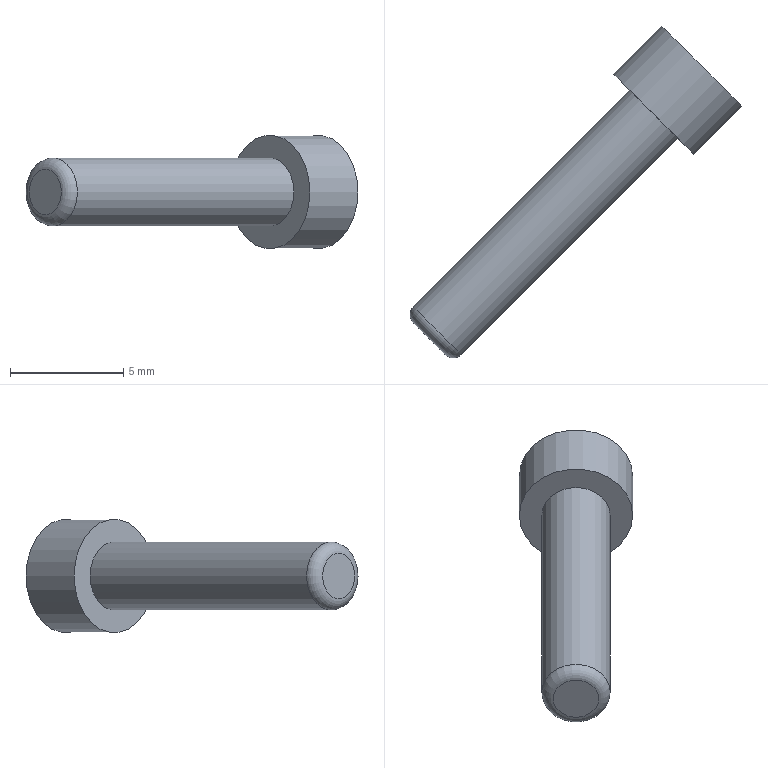Part | STEP file | gslz 2016.10.28-13_id650_x_t | 1 solid | 6 faces | box 14.642 x 14.642 x 5 mm | volume 157.397 mm3 | plane 3 | cylinder 2 | torus 1 | commonest cylinder face diameters 3 x1 5 x1
STEP:
#1=CARTESIAN_POINT('',(0.,0.,0.));
#2=DIRECTION('',(0.,0.,1.));
#3=DIRECTION('',(1.,0.,0.));
#4=AXIS2_PLACEMENT_3D('',#1,#2,#3);
#5=CARTESIAN_POINT('',(550.913,157.257,-21.226));
#6=VERTEX_POINT('',#5);
#7=CARTESIAN_POINT('',(551.974,156.197,-21.226));
#8=DIRECTION('',(0.7071,0.7071,0.));
#9=DIRECTION('',(-0.7071,0.7071,0.));
#10=AXIS2_PLACEMENT_3D('',#7,#8,#9);
#11=CIRCLE('',#10,1.5);
#12=CARTESIAN_POINT('',(552.328,156.55,-21.226));
#13=DIRECTION('',(0.7071,0.7071,0.));
#14=DIRECTION('',(-0.7071,0.7071,0.));
#15=AXIS2_PLACEMENT_3D('',#12,#13,#14);
#16=CYLINDRICAL_SURFACE('',#15,1.5);
#17=CARTESIAN_POINT('',(0.,-0.5));
#18=DIRECTION('',(1.,0.));
#19=VECTOR('',#18,1.);
#20=LINE('',#17,#19);
#21=(GEOMETRIC_REPRESENTATION_CONTEXT(2)PARAMETRIC_REPRESENTATION_CONTEXT()REPRESENTATION_CONTEXT('',''));
#22=DEFINITIONAL_REPRESENTATION('',(#20),#21);
#23=PCURVE('',#16,#22);
#24=CARTESIAN_POINT('',(551.974,156.197,-21.226));
#25=DIRECTION('',(0.7071,0.7071,0.));
#26=DIRECTION('',(-0.7071,0.7071,0.));
#27=AXIS2_PLACEMENT_3D('',#24,#25,#26);
#28=TOROIDAL_SURFACE('',#27,1.,0.5);
#29=CARTESIAN_POINT('',(0.,6.283));
#30=DIRECTION('',(1.,0.));
#31=VECTOR('',#30,1.);
#32=LINE('',#29,#31);
#33=(GEOMETRIC_REPRESENTATION_CONTEXT(2)PARAMETRIC_REPRESENTATION_CONTEXT()REPRESENTATION_CONTEXT('',''));
#34=DEFINITIONAL_REPRESENTATION('',(#32),#33);
#35=PCURVE('',#28,#34);
#36=SURFACE_CURVE('',#11,(#23,#35),.PCURVE_S1.);
#37=EDGE_CURVE('',#6,#6,#36,.T.);
#38=ORIENTED_EDGE('',*,*,#37,.T.);
#39=CARTESIAN_POINT('',(560.459,166.803,-21.226));
#40=VERTEX_POINT('',#39);
#41=CARTESIAN_POINT('',(550.913,157.257,-21.226));
#42=CARTESIAN_POINT('',(560.459,166.803,-21.226));
#43=B_SPLINE_CURVE_WITH_KNOTS('',1,(#41,#42),.UNSPECIFIED.,.F.,.F.,(2,2),(-0.5,13.),.PIECEWISE_BEZIER_KNOTS.);
#44=CARTESIAN_POINT('',(6.283,0.));
#45=DIRECTION('',(0.,1.));
#46=VECTOR('',#45,1.);
#47=LINE('',#44,#46);
#48=(GEOMETRIC_REPRESENTATION_CONTEXT(2)PARAMETRIC_REPRESENTATION_CONTEXT()REPRESENTATION_CONTEXT('',''));
#49=DEFINITIONAL_REPRESENTATION('',(#47),#48);
#50=PCURVE('',#16,#49);
#51=CARTESIAN_POINT('',(0.,0.));
#52=DIRECTION('',(0.,1.));
#53=VECTOR('',#52,1.);
#54=LINE('',#51,#53);
#55=(GEOMETRIC_REPRESENTATION_CONTEXT(2)PARAMETRIC_REPRESENTATION_CONTEXT()REPRESENTATION_CONTEXT('',''));
#56=DEFINITIONAL_REPRESENTATION('',(#54),#55);
#57=PCURVE('',#16,#56);
#58=SEAM_CURVE('',#43,(#50,#57),.PCURVE_S1.);
#59=EDGE_CURVE('',#6,#40,#58,.T.);
#60=ORIENTED_EDGE('',*,*,#59,.T.);
#61=CARTESIAN_POINT('',(561.52,165.743,-21.226));
#62=DIRECTION('',(0.7071,0.7071,0.));
#63=DIRECTION('',(-0.7071,0.7071,0.));
#64=AXIS2_PLACEMENT_3D('',#61,#62,#63);
#65=CIRCLE('',#64,1.5);
#66=CARTESIAN_POINT('',(0.,13.));
#67=DIRECTION('',(1.,0.));
#68=VECTOR('',#67,1.);
#69=LINE('',#66,#68);
#70=(GEOMETRIC_REPRESENTATION_CONTEXT(2)PARAMETRIC_REPRESENTATION_CONTEXT()REPRESENTATION_CONTEXT('',''));
#71=DEFINITIONAL_REPRESENTATION('',(#69),#70);
#72=PCURVE('',#16,#71);
#73=CARTESIAN_POINT('',(561.52,165.743,-21.226));
#74=DIRECTION('',(0.7071,0.7071,0.));
#75=DIRECTION('',(-0.7071,0.7071,0.));
#76=AXIS2_PLACEMENT_3D('',#73,#74,#75);
#77=PLANE('',#76);
#78=CARTESIAN_POINT('',(0.,0.));
#79=DIRECTION('',(1.,0.));
#80=AXIS2_PLACEMENT_2D('',#78,#79);
#81=CIRCLE('',#80,1.5);
#82=(GEOMETRIC_REPRESENTATION_CONTEXT(2)PARAMETRIC_REPRESENTATION_CONTEXT()REPRESENTATION_CONTEXT('',''));
#83=DEFINITIONAL_REPRESENTATION('',(#81),#82);
#84=PCURVE('',#77,#83);
#85=SURFACE_CURVE('',#65,(#72,#84),.PCURVE_S1.);
#86=EDGE_CURVE('',#40,#40,#85,.T.);
#87=ORIENTED_EDGE('',*,*,#86,.F.);
#88=ORIENTED_EDGE('',*,*,#59,.F.);
#89=EDGE_LOOP('',(#38,#60,#87,#88));
#90=FACE_BOUND('',#89,.T.);
#91=ADVANCED_FACE('',(#90),#16,.T.);
#92=CARTESIAN_POINT('',(550.913,156.55,-21.226));
#93=VERTEX_POINT('',#92);
#94=CARTESIAN_POINT('',(551.621,155.843,-21.226));
#95=DIRECTION('',(-0.7071,-0.7071,0.));
#96=DIRECTION('',(-0.7071,0.7071,0.));
#97=AXIS2_PLACEMENT_3D('',#94,#95,#96);
#98=CIRCLE('',#97,1.);
#99=CARTESIAN_POINT('',(551.621,155.843,-21.226));
#100=DIRECTION('',(0.7071,0.7071,0.));
#101=DIRECTION('',(-0.7071,0.7071,0.));
#102=AXIS2_PLACEMENT_3D('',#99,#100,#101);
#103=PLANE('',#102);
#104=CARTESIAN_POINT('',(1.,0.));
#105=CARTESIAN_POINT('',(1.,-1.732));
#106=CARTESIAN_POINT('',(-0.5,-0.866));
#107=CARTESIAN_POINT('',(-2.,0.));
#108=CARTESIAN_POINT('',(-0.5,0.866));
#109=CARTESIAN_POINT('',(1.,1.732));
#110=CARTESIAN_POINT('',(1.,0.));
#111=(BOUNDED_CURVE()B_SPLINE_CURVE(2,(#104,#105,#106,#107,#108,#109,#110),.UNSPECIFIED.,.T.,.F.)B_SPLINE_CURVE_WITH_KNOTS((1,2,2,2,2,1),(-2.094,0.,2.094,4.189,6.283,8.378),.UNSPECIFIED.)CURVE()GEOMETRIC_REPRESENTATION_ITEM()RATIONAL_B_SPLINE_CURVE((1.,0.5,1.,0.5,1.,0.5,1.))REPRESENTATION_ITEM(''));
#112=(GEOMETRIC_REPRESENTATION_CONTEXT(2)PARAMETRIC_REPRESENTATION_CONTEXT()REPRESENTATION_CONTEXT('',''));
#113=DEFINITIONAL_REPRESENTATION('',(#111),#112);
#114=PCURVE('',#103,#113);
#115=CARTESIAN_POINT('',(6.283,4.712));
#116=DIRECTION('',(-1.,0.));
#117=VECTOR('',#116,1.);
#118=LINE('',#115,#117);
#119=(GEOMETRIC_REPRESENTATION_CONTEXT(2)PARAMETRIC_REPRESENTATION_CONTEXT()REPRESENTATION_CONTEXT('',''));
#120=DEFINITIONAL_REPRESENTATION('',(#118),#119);
#121=PCURVE('',#28,#120);
#122=SURFACE_CURVE('',#98,(#114,#121),.PCURVE_S1.);
#123=EDGE_CURVE('',#93,#93,#122,.T.);
#124=ORIENTED_EDGE('',*,*,#123,.T.);
#125=EDGE_LOOP('',(#124));
#126=FACE_BOUND('',#125,.T.);
#127=ADVANCED_FACE('',(#126),#103,.F.);
#128=ORIENTED_EDGE('',*,*,#123,.F.);
#129=CARTESIAN_POINT('',(550.913,156.55,-21.226));
#130=CARTESIAN_POINT('',(550.819,156.645,-21.226));
#131=CARTESIAN_POINT('',(550.757,156.767,-21.226));
#132=CARTESIAN_POINT('',(550.735,156.904,-21.226));
#133=CARTESIAN_POINT('',(550.757,157.041,-21.226));
#134=CARTESIAN_POINT('',(550.819,157.163,-21.226));
#135=CARTESIAN_POINT('',(550.913,157.257,-21.226));
#136=(BOUNDED_CURVE()B_SPLINE_CURVE(6,(#129,#130,#131,#132,#133,#134,#135),.UNSPECIFIED.,.F.,.F.)B_SPLINE_CURVE_WITH_KNOTS((7,7),(4.712,6.283),.PIECEWISE_BEZIER_KNOTS.)CURVE()GEOMETRIC_REPRESENTATION_ITEM()RATIONAL_B_SPLINE_CURVE((1.031,1.01,0.9979,0.994,0.9979,1.01,1.031))REPRESENTATION_ITEM(''));
#137=CARTESIAN_POINT('',(6.283,0.));
#138=DIRECTION('',(0.,1.));
#139=VECTOR('',#138,1.);
#140=LINE('',#137,#139);
#141=(GEOMETRIC_REPRESENTATION_CONTEXT(2)PARAMETRIC_REPRESENTATION_CONTEXT()REPRESENTATION_CONTEXT('',''));
#142=DEFINITIONAL_REPRESENTATION('',(#140),#141);
#143=PCURVE('',#28,#142);
#144=CARTESIAN_POINT('',(0.,0.));
#145=DIRECTION('',(0.,1.));
#146=VECTOR('',#145,1.);
#147=LINE('',#144,#146);
#148=(GEOMETRIC_REPRESENTATION_CONTEXT(2)PARAMETRIC_REPRESENTATION_CONTEXT()REPRESENTATION_CONTEXT('',''));
#149=DEFINITIONAL_REPRESENTATION('',(#147),#148);
#150=PCURVE('',#28,#149);
#151=SEAM_CURVE('',#136,(#143,#150),.PCURVE_S1.);
#152=EDGE_CURVE('',#93,#6,#151,.T.);
#153=ORIENTED_EDGE('',*,*,#152,.T.);
#154=ORIENTED_EDGE('',*,*,#37,.F.);
#155=ORIENTED_EDGE('',*,*,#152,.F.);
#156=EDGE_LOOP('',(#128,#153,#154,#155));
#157=FACE_BOUND('',#156,.T.);
#158=ADVANCED_FACE('',(#157),#28,.T.);
#159=CARTESIAN_POINT('',(559.752,167.51,-21.226));
#160=VERTEX_POINT('',#159);
#161=CARTESIAN_POINT('',(561.52,165.743,-21.226));
#162=DIRECTION('',(0.7071,0.7071,0.));
#163=DIRECTION('',(-0.7071,0.7071,0.));
#164=AXIS2_PLACEMENT_3D('',#161,#162,#163);
#165=CIRCLE('',#164,2.5);
#166=CARTESIAN_POINT('',(0.,0.));
#167=DIRECTION('',(1.,0.));
#168=AXIS2_PLACEMENT_2D('',#166,#167);
#169=CIRCLE('',#168,2.5);
#170=(GEOMETRIC_REPRESENTATION_CONTEXT(2)PARAMETRIC_REPRESENTATION_CONTEXT()REPRESENTATION_CONTEXT('',''));
#171=DEFINITIONAL_REPRESENTATION('',(#169),#170);
#172=PCURVE('',#77,#171);
#173=CARTESIAN_POINT('',(563.641,167.864,-21.226));
#174=DIRECTION('',(-0.7071,-0.7071,0.));
#175=DIRECTION('',(0.7071,-0.7071,0.));
#176=AXIS2_PLACEMENT_3D('',#173,#174,#175);
#177=CYLINDRICAL_SURFACE('',#176,2.5);
#178=CARTESIAN_POINT('',(9.425,3.));
#179=DIRECTION('',(-1.,0.));
#180=VECTOR('',#179,1.);
#181=LINE('',#178,#180);
#182=(GEOMETRIC_REPRESENTATION_CONTEXT(2)PARAMETRIC_REPRESENTATION_CONTEXT()REPRESENTATION_CONTEXT('',''));
#183=DEFINITIONAL_REPRESENTATION('',(#181),#182);
#184=PCURVE('',#177,#183);
#185=SURFACE_CURVE('',#165,(#172,#184),.PCURVE_S1.);
#186=EDGE_CURVE('',#160,#160,#185,.T.);
#187=ORIENTED_EDGE('',*,*,#186,.F.);
#188=EDGE_LOOP('',(#187));
#189=FACE_BOUND('',#188,.T.);
#190=ORIENTED_EDGE('',*,*,#86,.T.);
#191=EDGE_LOOP('',(#190));
#192=FACE_BOUND('',#191,.T.);
#193=ADVANCED_FACE('',(#189,#192),#77,.F.);
#194=CARTESIAN_POINT('',(561.874,169.632,-21.226));
#195=VERTEX_POINT('',#194);
#196=CARTESIAN_POINT('',(563.641,167.864,-21.226));
#197=DIRECTION('',(0.7071,0.7071,0.));
#198=DIRECTION('',(-0.7071,0.7071,0.));
#199=AXIS2_PLACEMENT_3D('',#196,#197,#198);
#200=CIRCLE('',#199,2.5);
#201=CARTESIAN_POINT('',(9.425,0.));
#202=DIRECTION('',(-1.,0.));
#203=VECTOR('',#202,1.);
#204=LINE('',#201,#203);
#205=(GEOMETRIC_REPRESENTATION_CONTEXT(2)PARAMETRIC_REPRESENTATION_CONTEXT()REPRESENTATION_CONTEXT('',''));
#206=DEFINITIONAL_REPRESENTATION('',(#204),#205);
#207=PCURVE('',#177,#206);
#208=CARTESIAN_POINT('',(563.641,167.864,-21.226));
#209=DIRECTION('',(0.7071,0.7071,0.));
#210=DIRECTION('',(-0.7071,0.7071,0.));
#211=AXIS2_PLACEMENT_3D('',#208,#209,#210);
#212=PLANE('',#211);
#213=CARTESIAN_POINT('',(0.,0.));
#214=DIRECTION('',(1.,0.));
#215=AXIS2_PLACEMENT_2D('',#213,#214);
#216=CIRCLE('',#215,2.5);
#217=(GEOMETRIC_REPRESENTATION_CONTEXT(2)PARAMETRIC_REPRESENTATION_CONTEXT()REPRESENTATION_CONTEXT('',''));
#218=DEFINITIONAL_REPRESENTATION('',(#216),#217);
#219=PCURVE('',#212,#218);
#220=SURFACE_CURVE('',#200,(#207,#219),.PCURVE_S1.);
#221=EDGE_CURVE('',#195,#195,#220,.T.);
#222=ORIENTED_EDGE('',*,*,#221,.F.);
#223=CARTESIAN_POINT('',(561.874,169.632,-21.226));
#224=CARTESIAN_POINT('',(559.752,167.51,-21.226));
#225=B_SPLINE_CURVE_WITH_KNOTS('',1,(#223,#224),.UNSPECIFIED.,.F.,.F.,(2,2),(0.,3.),.PIECEWISE_BEZIER_KNOTS.);
#226=CARTESIAN_POINT('',(9.425,0.));
#227=DIRECTION('',(0.,1.));
#228=VECTOR('',#227,1.);
#229=LINE('',#226,#228);
#230=(GEOMETRIC_REPRESENTATION_CONTEXT(2)PARAMETRIC_REPRESENTATION_CONTEXT()REPRESENTATION_CONTEXT('',''));
#231=DEFINITIONAL_REPRESENTATION('',(#229),#230);
#232=PCURVE('',#177,#231);
#233=CARTESIAN_POINT('',(3.142,0.));
#234=DIRECTION('',(0.,1.));
#235=VECTOR('',#234,1.);
#236=LINE('',#233,#235);
#237=(GEOMETRIC_REPRESENTATION_CONTEXT(2)PARAMETRIC_REPRESENTATION_CONTEXT()REPRESENTATION_CONTEXT('',''));
#238=DEFINITIONAL_REPRESENTATION('',(#236),#237);
#239=PCURVE('',#177,#238);
#240=SEAM_CURVE('',#225,(#232,#239),.PCURVE_S1.);
#241=EDGE_CURVE('',#195,#160,#240,.T.);
#242=ORIENTED_EDGE('',*,*,#241,.T.);
#243=ORIENTED_EDGE('',*,*,#186,.T.);
#244=ORIENTED_EDGE('',*,*,#241,.F.);
#245=EDGE_LOOP('',(#222,#242,#243,#244));
#246=FACE_BOUND('',#245,.T.);
#247=ADVANCED_FACE('',(#246),#177,.T.);
#248=ORIENTED_EDGE('',*,*,#221,.T.);
#249=EDGE_LOOP('',(#248));
#250=FACE_BOUND('',#249,.T.);
#251=ADVANCED_FACE('',(#250),#212,.T.);
#252=CLOSED_SHELL('',(#91,#127,#158,#193,#247,#251));
#253=MANIFOLD_SOLID_BREP('',#252);
#254=(LENGTH_UNIT()NAMED_UNIT(*)SI_UNIT(.MILLI.,.METRE.));
#255=UNCERTAINTY_MEASURE_WITH_UNIT(LENGTH_MEASURE(0.00001),#254,'','');
#256=(NAMED_UNIT(*)PLANE_ANGLE_UNIT()SI_UNIT($,.RADIAN.));
#257=(NAMED_UNIT(*)SI_UNIT($,.STERADIAN.)SOLID_ANGLE_UNIT());
#258=(GEOMETRIC_REPRESENTATION_CONTEXT(3)GLOBAL_UNCERTAINTY_ASSIGNED_CONTEXT((#255))GLOBAL_UNIT_ASSIGNED_CONTEXT((#254,#256,#257))REPRESENTATION_CONTEXT('',''));
#259=ADVANCED_BREP_SHAPE_REPRESENTATION('',(#4,#253),#258);